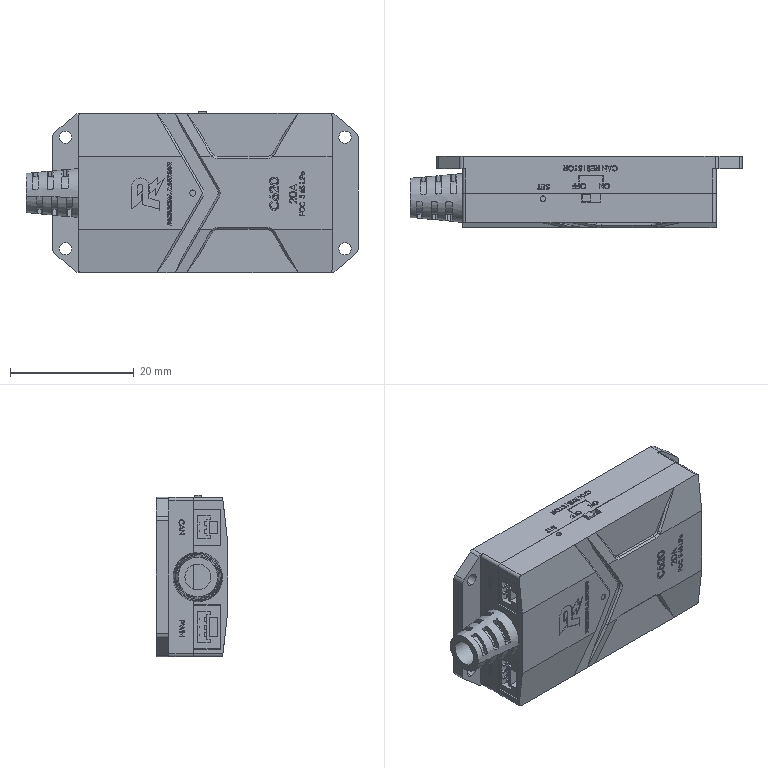Part | SolidWorks | features BaseBody 18 | 18 solids | 1656 faces | box 53.7 x 11.5 x 26.125 mm | volume 11767 mm3 | plane 897 | spline 425 | cylinder 266 | torus 60 | cone 8 | commonest cylinder face diameters 0.2 x112 0.4 x48 2 x35 3 x16 1 x14 5.3 x12